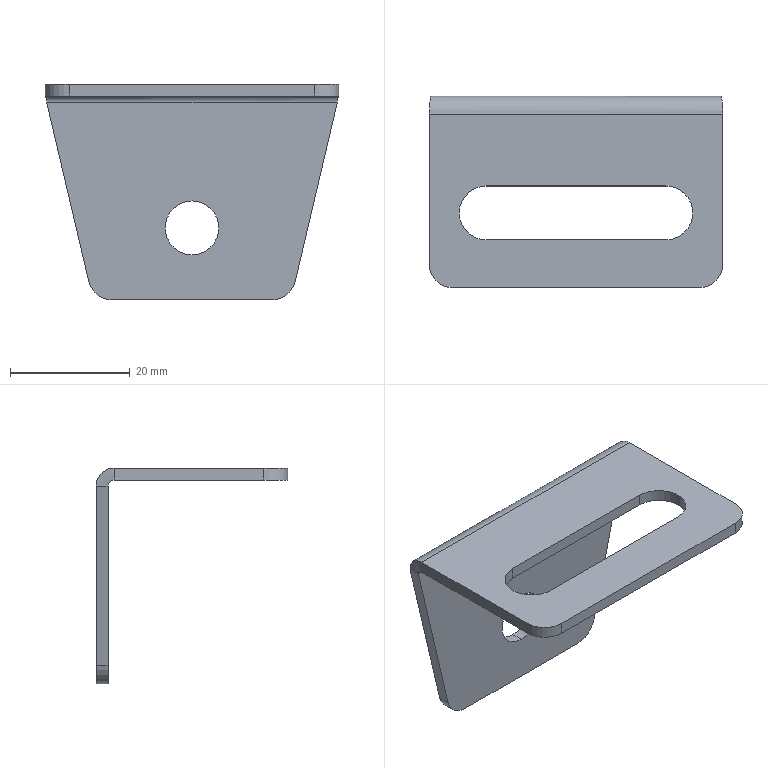Part | STEP file | 1.6米托片 | 1 solid | 25 faces | box 49 x 32 x 36 mm | volume 5023 mm3 | plane 12 | cylinder 11 | spline 2 | commonest cylinder face diameters 9 x5 8 x4 2 x1 6 x1
STEP:
#1=CARTESIAN_POINT('',(5.,12.5,2.));
#2=VERTEX_POINT('',#1);
#3=CARTESIAN_POINT('',(9.5,17.,2.));
#4=VERTEX_POINT('',#3);
#5=CARTESIAN_POINT('',(9.5,12.5,2.));
#6=DIRECTION('',(0.,0.,-1.));
#7=DIRECTION('',(-1.,0.,0.));
#8=AXIS2_PLACEMENT_3D('',#5,#6,#7);
#9=CIRCLE('',#8,4.5);
#10=EDGE_CURVE('',#2,#4,#9,.T.);
#11=ORIENTED_EDGE('',*,*,#10,.F.);
#12=CARTESIAN_POINT('',(5.,12.5,0.));
#13=VERTEX_POINT('',#12);
#14=CARTESIAN_POINT('',(5.,12.5,10.));
#15=DIRECTION('',(0.,0.,-1.));
#16=VECTOR('',#15,1000.);
#17=LINE('',#14,#16);
#18=EDGE_CURVE('',#2,#13,#17,.T.);
#19=ORIENTED_EDGE('',*,*,#18,.T.);
#20=CARTESIAN_POINT('',(9.5,17.,0.));
#21=VERTEX_POINT('',#20);
#22=CARTESIAN_POINT('',(9.5,12.5,0.));
#23=DIRECTION('',(0.,0.,-1.));
#24=DIRECTION('',(-1.,0.,0.));
#25=AXIS2_PLACEMENT_3D('',#22,#23,#24);
#26=CIRCLE('',#25,4.5);
#27=EDGE_CURVE('',#13,#21,#26,.T.);
#28=ORIENTED_EDGE('',*,*,#27,.T.);
#29=CARTESIAN_POINT('',(9.5,17.,10.));
#30=DIRECTION('',(0.,0.,-1.));
#31=VECTOR('',#30,1000.);
#32=LINE('',#29,#31);
#33=EDGE_CURVE('',#4,#21,#32,.T.);
#34=ORIENTED_EDGE('',*,*,#33,.F.);
#35=EDGE_LOOP('',(#11,#19,#28,#34));
#36=FACE_OUTER_BOUND('',#35,.T.);
#37=CARTESIAN_POINT('',(9.5,12.5,10.));
#38=DIRECTION('',(0.,0.,-1.));
#39=DIRECTION('',(-1.,0.,0.));
#40=AXIS2_PLACEMENT_3D('',#37,#38,#39);
#41=CYLINDRICAL_SURFACE('',#40,4.5);
#42=ADVANCED_FACE('',(#36),#41,.F.);
#43=CARTESIAN_POINT('',(24.5,32.,-17.5));
#44=VERTEX_POINT('',#43);
#45=CARTESIAN_POINT('',(24.5,32.,-26.5));
#46=VERTEX_POINT('',#45);
#47=CARTESIAN_POINT('',(24.5,32.,-22.));
#48=DIRECTION('',(0.,-1.,0.));
#49=DIRECTION('',(0.,0.,-1.));
#50=AXIS2_PLACEMENT_3D('',#47,#48,#49);
#51=CIRCLE('',#50,4.5);
#52=EDGE_CURVE('',#44,#46,#51,.T.);
#53=ORIENTED_EDGE('',*,*,#52,.F.);
#54=CARTESIAN_POINT('',(24.5,30.,-17.5));
#55=VERTEX_POINT('',#54);
#56=CARTESIAN_POINT('',(24.5,40.,-17.5));
#57=DIRECTION('',(0.,-1.,0.));
#58=VECTOR('',#57,1000.);
#59=LINE('',#56,#58);
#60=EDGE_CURVE('',#44,#55,#59,.T.);
#61=ORIENTED_EDGE('',*,*,#60,.T.);
#62=CARTESIAN_POINT('',(24.5,30.,-26.5));
#63=VERTEX_POINT('',#62);
#64=CARTESIAN_POINT('',(24.5,30.,-22.));
#65=DIRECTION('',(0.,-1.,0.));
#66=DIRECTION('',(0.,0.,-1.));
#67=AXIS2_PLACEMENT_3D('',#64,#65,#66);
#68=CIRCLE('',#67,4.5);
#69=EDGE_CURVE('',#55,#63,#68,.T.);
#70=ORIENTED_EDGE('',*,*,#69,.T.);
#71=CARTESIAN_POINT('',(24.5,40.,-26.5));
#72=DIRECTION('',(0.,-1.,0.));
#73=VECTOR('',#72,1000.);
#74=LINE('',#71,#73);
#75=EDGE_CURVE('',#46,#63,#74,.T.);
#76=ORIENTED_EDGE('',*,*,#75,.F.);
#77=EDGE_LOOP('',(#53,#61,#70,#76));
#78=FACE_OUTER_BOUND('',#77,.T.);
#79=CARTESIAN_POINT('',(24.5,40.,-22.));
#80=DIRECTION('',(0.,-1.,0.));
#81=DIRECTION('',(0.,0.,-1.));
#82=AXIS2_PLACEMENT_3D('',#79,#80,#81);
#83=CYLINDRICAL_SURFACE('',#82,4.5);
#84=ADVANCED_FACE('',(#78),#83,.F.);
#85=CARTESIAN_POINT('',(39.5,17.,2.));
#86=VERTEX_POINT('',#85);
#87=CARTESIAN_POINT('',(0.,17.,2.));
#88=DIRECTION('',(1.,0.,0.));
#89=VECTOR('',#88,1000.);
#90=LINE('',#87,#89);
#91=EDGE_CURVE('',#4,#86,#90,.T.);
#92=ORIENTED_EDGE('',*,*,#91,.T.);
#93=CARTESIAN_POINT('',(39.5,8.,2.));
#94=VERTEX_POINT('',#93);
#95=CARTESIAN_POINT('',(39.5,12.5,2.));
#96=DIRECTION('',(0.,0.,-1.));
#97=DIRECTION('',(-1.,0.,0.));
#98=AXIS2_PLACEMENT_3D('',#95,#96,#97);
#99=CIRCLE('',#98,4.5);
#100=EDGE_CURVE('',#86,#94,#99,.T.);
#101=ORIENTED_EDGE('',*,*,#100,.T.);
#102=CARTESIAN_POINT('',(9.5,8.,2.));
#103=VERTEX_POINT('',#102);
#104=CARTESIAN_POINT('',(0.,8.,2.));
#105=DIRECTION('',(-1.,0.,0.));
#106=VECTOR('',#105,1000.);
#107=LINE('',#104,#106);
#108=EDGE_CURVE('',#94,#103,#107,.T.);
#109=ORIENTED_EDGE('',*,*,#108,.T.);
#110=CARTESIAN_POINT('',(9.5,12.5,2.));
#111=DIRECTION('',(0.,0.,-1.));
#112=DIRECTION('',(-1.,0.,0.));
#113=AXIS2_PLACEMENT_3D('',#110,#111,#112);
#114=CIRCLE('',#113,4.5);
#115=EDGE_CURVE('',#103,#2,#114,.T.);
#116=ORIENTED_EDGE('',*,*,#115,.T.);
#117=ORIENTED_EDGE('',*,*,#10,.T.);
#118=EDGE_LOOP('',(#92,#101,#109,#116,#117));
#119=FACE_BOUND('',#118,.T.);
#120=CARTESIAN_POINT('',(4.,0.,2.));
#121=VERTEX_POINT('',#120);
#122=CARTESIAN_POINT('',(45.,0.,2.));
#123=VERTEX_POINT('',#122);
#124=CARTESIAN_POINT('',(0.,0.,2.));
#125=DIRECTION('',(1.,0.,0.));
#126=VECTOR('',#125,1000.);
#127=LINE('',#124,#126);
#128=EDGE_CURVE('',#121,#123,#127,.T.);
#129=ORIENTED_EDGE('',*,*,#128,.T.);
#130=CARTESIAN_POINT('',(49.,4.,2.));
#131=VERTEX_POINT('',#130);
#132=CARTESIAN_POINT('',(45.,4.,2.));
#133=DIRECTION('',(0.,0.,1.));
#134=DIRECTION('',(-1.,0.,0.));
#135=AXIS2_PLACEMENT_3D('',#132,#133,#134);
#136=CIRCLE('',#135,4.);
#137=EDGE_CURVE('',#123,#131,#136,.T.);
#138=ORIENTED_EDGE('',*,*,#137,.T.);
#139=CARTESIAN_POINT('',(49.,29.,2.));
#140=VERTEX_POINT('',#139);
#141=CARTESIAN_POINT('',(49.,32.,2.));
#142=DIRECTION('',(0.,-1.,0.));
#143=VECTOR('',#142,1000.);
#144=LINE('',#141,#143);
#145=EDGE_CURVE('',#140,#131,#144,.T.);
#146=ORIENTED_EDGE('',*,*,#145,.F.);
#147=CARTESIAN_POINT('',(0.,29.,2.));
#148=VERTEX_POINT('',#147);
#149=CARTESIAN_POINT('',(49.,29.,2.));
#150=DIRECTION('',(-1.,0.,0.));
#151=VECTOR('',#150,1000.);
#152=LINE('',#149,#151);
#153=EDGE_CURVE('',#140,#148,#152,.T.);
#154=ORIENTED_EDGE('',*,*,#153,.T.);
#155=CARTESIAN_POINT('',(0.,4.,2.));
#156=VERTEX_POINT('',#155);
#157=CARTESIAN_POINT('',(0.,32.,2.));
#158=DIRECTION('',(0.,-1.,0.));
#159=VECTOR('',#158,1000.);
#160=LINE('',#157,#159);
#161=EDGE_CURVE('',#148,#156,#160,.T.);
#162=ORIENTED_EDGE('',*,*,#161,.T.);
#163=CARTESIAN_POINT('',(4.,4.,2.));
#164=DIRECTION('',(0.,0.,1.));
#165=DIRECTION('',(-1.,0.,0.));
#166=AXIS2_PLACEMENT_3D('',#163,#164,#165);
#167=CIRCLE('',#166,4.);
#168=EDGE_CURVE('',#156,#121,#167,.T.);
#169=ORIENTED_EDGE('',*,*,#168,.T.);
#170=EDGE_LOOP('',(#129,#138,#146,#154,#162,#169));
#171=FACE_OUTER_BOUND('',#170,.T.);
#172=CARTESIAN_POINT('',(0.,32.,2.));
#173=DIRECTION('',(0.,0.,-1.));
#174=DIRECTION('',(-1.,0.,0.));
#175=AXIS2_PLACEMENT_3D('',#172,#173,#174);
#176=PLANE('',#175);
#177=ADVANCED_FACE('',(#119,#171),#176,.F.);
#178=ORIENTED_EDGE('',*,*,#145,.T.);
#179=CARTESIAN_POINT('',(49.,4.,0.));
#180=VERTEX_POINT('',#179);
#181=CARTESIAN_POINT('',(49.,4.,0.));
#182=DIRECTION('',(0.,0.,-1.));
#183=VECTOR('',#182,1000.);
#184=LINE('',#181,#183);
#185=EDGE_CURVE('',#131,#180,#184,.T.);
#186=ORIENTED_EDGE('',*,*,#185,.T.);
#187=CARTESIAN_POINT('',(49.,29.,0.));
#188=VERTEX_POINT('',#187);
#189=CARTESIAN_POINT('',(49.,32.,0.));
#190=DIRECTION('',(0.,-1.,0.));
#191=VECTOR('',#190,1000.);
#192=LINE('',#189,#191);
#193=EDGE_CURVE('',#188,#180,#192,.T.);
#194=ORIENTED_EDGE('',*,*,#193,.F.);
#195=CARTESIAN_POINT('',(49.,29.,0.));
#196=DIRECTION('',(0.,0.,1.));
#197=VECTOR('',#196,1000.);
#198=LINE('',#195,#197);
#199=EDGE_CURVE('',#188,#140,#198,.T.);
#200=ORIENTED_EDGE('',*,*,#199,.T.);
#201=EDGE_LOOP('',(#178,#186,#194,#200));
#202=FACE_OUTER_BOUND('',#201,.T.);
#203=CARTESIAN_POINT('',(49.,32.,0.));
#204=DIRECTION('',(1.,0.,0.));
#205=DIRECTION('',(0.,0.,-1.));
#206=AXIS2_PLACEMENT_3D('',#203,#204,#205);
#207=PLANE('',#206);
#208=ADVANCED_FACE('',(#202),#207,.T.);
#209=CARTESIAN_POINT('',(39.5,17.,0.));
#210=VERTEX_POINT('',#209);
#211=CARTESIAN_POINT('',(39.5,8.,0.));
#212=VERTEX_POINT('',#211);
#213=CARTESIAN_POINT('',(39.5,12.5,0.));
#214=DIRECTION('',(0.,0.,-1.));
#215=DIRECTION('',(-1.,0.,0.));
#216=AXIS2_PLACEMENT_3D('',#213,#214,#215);
#217=CIRCLE('',#216,4.5);
#218=EDGE_CURVE('',#210,#212,#217,.T.);
#219=ORIENTED_EDGE('',*,*,#218,.F.);
#220=CARTESIAN_POINT('',(39.5,17.,0.));
#221=DIRECTION('',(1.,0.,0.));
#222=VECTOR('',#221,1000.);
#223=LINE('',#220,#222);
#224=EDGE_CURVE('',#21,#210,#223,.T.);
#225=ORIENTED_EDGE('',*,*,#224,.F.);
#226=ORIENTED_EDGE('',*,*,#27,.F.);
#227=CARTESIAN_POINT('',(9.5,8.,0.));
#228=VERTEX_POINT('',#227);
#229=CARTESIAN_POINT('',(9.5,12.5,0.));
#230=DIRECTION('',(0.,0.,-1.));
#231=DIRECTION('',(-1.,0.,0.));
#232=AXIS2_PLACEMENT_3D('',#229,#230,#231);
#233=CIRCLE('',#232,4.5);
#234=EDGE_CURVE('',#228,#13,#233,.T.);
#235=ORIENTED_EDGE('',*,*,#234,.F.);
#236=CARTESIAN_POINT('',(39.5,8.,0.));
#237=DIRECTION('',(-1.,0.,0.));
#238=VECTOR('',#237,1000.);
#239=LINE('',#236,#238);
#240=EDGE_CURVE('',#212,#228,#239,.T.);
#241=ORIENTED_EDGE('',*,*,#240,.F.);
#242=EDGE_LOOP('',(#219,#225,#226,#235,#241));
#243=FACE_BOUND('',#242,.T.);
#244=ORIENTED_EDGE('',*,*,#193,.T.);
#245=CARTESIAN_POINT('',(45.,0.,0.));
#246=VERTEX_POINT('',#245);
#247=CARTESIAN_POINT('',(45.,4.,0.));
#248=DIRECTION('',(0.,0.,-1.));
#249=DIRECTION('',(-1.,0.,0.));
#250=AXIS2_PLACEMENT_3D('',#247,#248,#249);
#251=CIRCLE('',#250,4.);
#252=EDGE_CURVE('',#180,#246,#251,.T.);
#253=ORIENTED_EDGE('',*,*,#252,.T.);
#254=CARTESIAN_POINT('',(4.,0.,0.));
#255=VERTEX_POINT('',#254);
#256=CARTESIAN_POINT('',(0.,0.,0.));
#257=DIRECTION('',(1.,0.,0.));
#258=VECTOR('',#257,1000.);
#259=LINE('',#256,#258);
#260=EDGE_CURVE('',#255,#246,#259,.T.);
#261=ORIENTED_EDGE('',*,*,#260,.F.);
#262=CARTESIAN_POINT('',(0.,4.,0.));
#263=VERTEX_POINT('',#262);
#264=CARTESIAN_POINT('',(4.,4.,0.));
#265=DIRECTION('',(0.,0.,-1.));
#266=DIRECTION('',(-1.,0.,0.));
#267=AXIS2_PLACEMENT_3D('',#264,#265,#266);
#268=CIRCLE('',#267,4.);
#269=EDGE_CURVE('',#255,#263,#268,.T.);
#270=ORIENTED_EDGE('',*,*,#269,.T.);
#271=CARTESIAN_POINT('',(0.,29.,0.));
#272=VERTEX_POINT('',#271);
#273=CARTESIAN_POINT('',(0.,32.,0.));
#274=DIRECTION('',(0.,-1.,0.));
#275=VECTOR('',#274,1000.);
#276=LINE('',#273,#275);
#277=EDGE_CURVE('',#272,#263,#276,.T.);
#278=ORIENTED_EDGE('',*,*,#277,.F.);
#279=CARTESIAN_POINT('',(49.,29.,0.));
#280=DIRECTION('',(-1.,0.,0.));
#281=VECTOR('',#280,1000.);
#282=LINE('',#279,#281);
#283=EDGE_CURVE('',#188,#272,#282,.T.);
#284=ORIENTED_EDGE('',*,*,#283,.F.);
#285=EDGE_LOOP('',(#244,#253,#261,#270,#278,#284));
#286=FACE_OUTER_BOUND('',#285,.T.);
#287=CARTESIAN_POINT('',(0.,32.,0.));
#288=DIRECTION('',(0.,0.,-1.));
#289=DIRECTION('',(-1.,0.,0.));
#290=AXIS2_PLACEMENT_3D('',#287,#288,#289);
#291=PLANE('',#290);
#292=ADVANCED_FACE('',(#243,#286),#291,.T.);
#293=ORIENTED_EDGE('',*,*,#277,.T.);
#294=CARTESIAN_POINT('',(0.,4.,2.));
#295=DIRECTION('',(0.,0.,1.));
#296=VECTOR('',#295,1000.);
#297=LINE('',#294,#296);
#298=EDGE_CURVE('',#263,#156,#297,.T.);
#299=ORIENTED_EDGE('',*,*,#298,.T.);
#300=ORIENTED_EDGE('',*,*,#161,.F.);
#301=CARTESIAN_POINT('',(0.,29.,0.));
#302=DIRECTION('',(0.,0.,1.));
#303=VECTOR('',#302,1000.);
#304=LINE('',#301,#303);
#305=EDGE_CURVE('',#272,#148,#304,.T.);
#306=ORIENTED_EDGE('',*,*,#305,.F.);
#307=EDGE_LOOP('',(#293,#299,#300,#306));
#308=FACE_OUTER_BOUND('',#307,.T.);
#309=CARTESIAN_POINT('',(0.,32.,2.));
#310=DIRECTION('',(-1.,0.,0.));
#311=DIRECTION('',(0.,0.,1.));
#312=AXIS2_PLACEMENT_3D('',#309,#310,#311);
#313=PLANE('',#312);
#314=ADVANCED_FACE('',(#308),#313,.T.);
#315=ORIENTED_EDGE('',*,*,#260,.T.);
#316=CARTESIAN_POINT('',(45.,0.,0.));
#317=DIRECTION('',(0.,0.,1.));
#318=VECTOR('',#317,1000.);
#319=LINE('',#316,#318);
#320=EDGE_CURVE('',#246,#123,#319,.T.);
#321=ORIENTED_EDGE('',*,*,#320,.T.);
#322=ORIENTED_EDGE('',*,*,#128,.F.);
#323=CARTESIAN_POINT('',(4.,0.,0.));
#324=DIRECTION('',(0.,0.,-1.));
#325=VECTOR('',#324,1000.);
#326=LINE('',#323,#325);
#327=EDGE_CURVE('',#121,#255,#326,.T.);
#328=ORIENTED_EDGE('',*,*,#327,.T.);
#329=EDGE_LOOP('',(#315,#321,#322,#328));
#330=FACE_OUTER_BOUND('',#329,.T.);
#331=CARTESIAN_POINT('',(0.,0.,0.));
#332=DIRECTION('',(0.,-1.,0.));
#333=DIRECTION('',(-1.,0.,0.));
#334=AXIS2_PLACEMENT_3D('',#331,#332,#333);
#335=PLANE('',#334);
#336=ADVANCED_FACE('',(#330),#335,.T.);
#337=CARTESIAN_POINT('',(0.2353,30.,-1.));
#338=VERTEX_POINT('',#337);
#339=CARTESIAN_POINT('',(0.2353,32.,-1.));
#340=VERTEX_POINT('',#339);
#341=CARTESIAN_POINT('',(0.2353,32.,-1.));
#342=DIRECTION('',(0.,1.,0.));
#343=VECTOR('',#342,1000.);
#344=LINE('',#341,#343);
#345=EDGE_CURVE('',#338,#340,#344,.T.);
#346=ORIENTED_EDGE('',*,*,#345,.F.);
#347=CARTESIAN_POINT('',(0.,29.,0.));
#348=CARTESIAN_POINT('',(0.03922,29.262,0.));
#349=CARTESIAN_POINT('',(0.07843,29.522,-0.1078));
#350=CARTESIAN_POINT('',(0.1569,29.892,-0.478));
#351=CARTESIAN_POINT('',(0.1961,30.,-0.7382));
#352=CARTESIAN_POINT('',(0.2353,30.,-1.));
#353=B_SPLINE_CURVE_WITH_KNOTS('',3,(#347,#348,#349,#350,#351,#352),.UNSPECIFIED.,.F.,.F.,(4,2,4),(0.,0.5,1.),.UNSPECIFIED.);
#354=EDGE_CURVE('',#272,#338,#353,.T.);
#355=ORIENTED_EDGE('',*,*,#354,.F.);
#356=ORIENTED_EDGE('',*,*,#305,.T.);
#357=CARTESIAN_POINT('',(0.,29.,2.));
#358=CARTESIAN_POINT('',(0.01961,29.393,2.));
#359=CARTESIAN_POINT('',(0.03922,29.785,1.922));
#360=CARTESIAN_POINT('',(0.07843,30.511,1.621));
#361=CARTESIAN_POINT('',(0.09804,30.844,1.399));
#362=CARTESIAN_POINT('',(0.1373,31.399,0.8436));
#363=CARTESIAN_POINT('',(0.1569,31.621,0.5109));
#364=CARTESIAN_POINT('',(0.1961,31.922,-0.2148));
#365=CARTESIAN_POINT('',(0.2157,32.,-0.6073));
#366=CARTESIAN_POINT('',(0.2353,32.,-1.));
#367=B_SPLINE_CURVE_WITH_KNOTS('',3,(#357,#358,#359,#360,#361,#362,#363,#364,#365,#366),.UNSPECIFIED.,.F.,.F.,(4,2,2,2,4),(0.,0.25,0.5,0.75,1.),.UNSPECIFIED.);
#368=EDGE_CURVE('',#148,#340,#367,.T.);
#369=ORIENTED_EDGE('',*,*,#368,.T.);
#370=EDGE_LOOP('',(#346,#355,#356,#369));
#371=FACE_OUTER_BOUND('',#370,.T.);
#372=CARTESIAN_POINT('',(0.,29.,2.02));
#373=CARTESIAN_POINT('',(0.01961,29.395,2.02));
#374=CARTESIAN_POINT('',(0.03922,29.79,1.941));
#375=CARTESIAN_POINT('',(0.07843,30.521,1.639));
#376=CARTESIAN_POINT('',(0.09804,30.856,1.415));
#377=CARTESIAN_POINT('',(0.1373,31.415,0.8559));
#378=CARTESIAN_POINT('',(0.1569,31.639,0.5209));
#379=CARTESIAN_POINT('',(0.1961,31.941,-0.2095));
#380=CARTESIAN_POINT('',(0.2157,32.02,-0.6046));
#381=CARTESIAN_POINT('',(0.2353,32.02,-1.));
#382=CARTESIAN_POINT('',(0.,29.,2.));
#383=CARTESIAN_POINT('',(0.01961,29.393,2.));
#384=CARTESIAN_POINT('',(0.03922,29.785,1.922));
#385=CARTESIAN_POINT('',(0.07843,30.511,1.621));
#386=CARTESIAN_POINT('',(0.09804,30.844,1.399));
#387=CARTESIAN_POINT('',(0.1373,31.399,0.8436));
#388=CARTESIAN_POINT('',(0.1569,31.621,0.5109));
#389=CARTESIAN_POINT('',(0.1961,31.922,-0.2148));
#390=CARTESIAN_POINT('',(0.2157,32.,-0.6072));
#391=CARTESIAN_POINT('',(0.2353,32.,-1.));
#392=CARTESIAN_POINT('',(0.,29.,0.));
#393=CARTESIAN_POINT('',(0.01961,29.131,0.));
#394=CARTESIAN_POINT('',(0.03922,29.262,-0.02603));
#395=CARTESIAN_POINT('',(0.07843,29.504,-0.1262));
#396=CARTESIAN_POINT('',(0.09804,29.615,-0.2003));
#397=CARTESIAN_POINT('',(0.1373,29.8,-0.3855));
#398=CARTESIAN_POINT('',(0.1569,29.874,-0.4964));
#399=CARTESIAN_POINT('',(0.1961,29.974,-0.7383));
#400=CARTESIAN_POINT('',(0.2157,30.,-0.8691));
#401=CARTESIAN_POINT('',(0.2353,30.,-1.));
#402=CARTESIAN_POINT('',(0.,29.,-0.0202));
#403=CARTESIAN_POINT('',(0.01961,29.128,-0.0202));
#404=CARTESIAN_POINT('',(0.03922,29.256,-0.0457));
#405=CARTESIAN_POINT('',(0.07843,29.493,-0.1439));
#406=CARTESIAN_POINT('',(0.09804,29.602,-0.2165));
#407=CARTESIAN_POINT('',(0.1373,29.784,-0.3979));
#408=CARTESIAN_POINT('',(0.1569,29.856,-0.5066));
#409=CARTESIAN_POINT('',(0.1961,29.954,-0.7435));
#410=CARTESIAN_POINT('',(0.2157,29.98,-0.8717));
#411=CARTESIAN_POINT('',(0.2353,29.98,-1.));
#412=B_SPLINE_SURFACE_WITH_KNOTS('',1,3,((#372,#373,#374,#375,#376,#377,#378,#379,#380,#381),(#382,#383,#384,#385,#386,#387,#388,#389,#390,#391),(#392,#393,#394,#395,#396,#397,#398,#399,#400,#401),(#402,#403,#404,#405,#406,#407,#408,#409,#410,#411)),.UNSPECIFIED.,.F.,.F.,.F.,(2,1,1,2),(4,2,2,2,4),(-0.01,0.,1.,1.01),(0.,0.25,0.5,0.75,1.),.UNSPECIFIED.);
#413=ADVANCED_FACE('',(#371),#412,.F.);
#414=CARTESIAN_POINT('',(48.765,30.,-1.));
#415=VERTEX_POINT('',#414);
#416=CARTESIAN_POINT('',(48.765,30.,-1.));
#417=CARTESIAN_POINT('',(48.804,30.,-0.7382));
#418=CARTESIAN_POINT('',(48.843,29.892,-0.478));
#419=CARTESIAN_POINT('',(48.922,29.522,-0.1078));
#420=CARTESIAN_POINT('',(48.961,29.262,0.));
#421=CARTESIAN_POINT('',(49.,29.,0.));
#422=B_SPLINE_CURVE_WITH_KNOTS('',3,(#416,#417,#418,#419,#420,#421),.UNSPECIFIED.,.F.,.F.,(4,2,4),(0.,0.5,1.),.UNSPECIFIED.);
#423=EDGE_CURVE('',#415,#188,#422,.T.);
#424=ORIENTED_EDGE('',*,*,#423,.F.);
#425=CARTESIAN_POINT('',(48.765,32.,-1.));
#426=VERTEX_POINT('',#425);
#427=CARTESIAN_POINT('',(48.765,30.,-1.));
#428=DIRECTION('',(0.,1.,0.));
#429=VECTOR('',#428,1000.);
#430=LINE('',#427,#429);
#431=EDGE_CURVE('',#415,#426,#430,.T.);
#432=ORIENTED_EDGE('',*,*,#431,.T.);
#433=CARTESIAN_POINT('',(48.765,32.,-1.));
#434=CARTESIAN_POINT('',(48.784,32.,-0.6073));
#435=CARTESIAN_POINT('',(48.804,31.922,-0.2148));
#436=CARTESIAN_POINT('',(48.843,31.621,0.5109));
#437=CARTESIAN_POINT('',(48.863,31.399,0.8436));
#438=CARTESIAN_POINT('',(48.902,30.844,1.399));
#439=CARTESIAN_POINT('',(48.922,30.511,1.621));
#440=CARTESIAN_POINT('',(48.961,29.785,1.922));
#441=CARTESIAN_POINT('',(48.98,29.393,2.));
#442=CARTESIAN_POINT('',(49.,29.,2.));
#443=B_SPLINE_CURVE_WITH_KNOTS('',3,(#433,#434,#435,#436,#437,#438,#439,#440,#441,#442),.UNSPECIFIED.,.F.,.F.,(4,2,2,2,4),(0.,0.25,0.5,0.75,1.),.UNSPECIFIED.);
#444=EDGE_CURVE('',#426,#140,#443,.T.);
#445=ORIENTED_EDGE('',*,*,#444,.T.);
#446=ORIENTED_EDGE('',*,*,#199,.F.);
#447=EDGE_LOOP('',(#424,#432,#445,#446));
#448=FACE_OUTER_BOUND('',#447,.T.);
#449=CARTESIAN_POINT('',(48.765,32.02,-1.));
#450=CARTESIAN_POINT('',(48.784,32.02,-0.6046));
#451=CARTESIAN_POINT('',(48.804,31.941,-0.2095));
#452=CARTESIAN_POINT('',(48.843,31.639,0.5209));
#453=CARTESIAN_POINT('',(48.863,31.415,0.8559));
#454=CARTESIAN_POINT('',(48.902,30.856,1.415));
#455=CARTESIAN_POINT('',(48.922,30.521,1.639));
#456=CARTESIAN_POINT('',(48.961,29.79,1.941));
#457=CARTESIAN_POINT('',(48.98,29.395,2.02));
#458=CARTESIAN_POINT('',(49.,29.,2.02));
#459=CARTESIAN_POINT('',(48.765,32.,-1.));
#460=CARTESIAN_POINT('',(48.784,32.,-0.6072));
#461=CARTESIAN_POINT('',(48.804,31.922,-0.2148));
#462=CARTESIAN_POINT('',(48.843,31.621,0.5109));
#463=CARTESIAN_POINT('',(48.863,31.399,0.8436));
#464=CARTESIAN_POINT('',(48.902,30.844,1.399));
#465=CARTESIAN_POINT('',(48.922,30.511,1.621));
#466=CARTESIAN_POINT('',(48.961,29.785,1.922));
#467=CARTESIAN_POINT('',(48.98,29.393,2.));
#468=CARTESIAN_POINT('',(49.,29.,2.));
#469=CARTESIAN_POINT('',(48.765,30.,-1.));
#470=CARTESIAN_POINT('',(48.784,30.,-0.8691));
#471=CARTESIAN_POINT('',(48.804,29.974,-0.7383));
#472=CARTESIAN_POINT('',(48.843,29.874,-0.4964));
#473=CARTESIAN_POINT('',(48.863,29.8,-0.3855));
#474=CARTESIAN_POINT('',(48.902,29.615,-0.2003));
#475=CARTESIAN_POINT('',(48.922,29.504,-0.1262));
#476=CARTESIAN_POINT('',(48.961,29.262,-0.02603));
#477=CARTESIAN_POINT('',(48.98,29.131,0.));
#478=CARTESIAN_POINT('',(49.,29.,0.));
#479=CARTESIAN_POINT('',(48.765,29.98,-1.));
#480=CARTESIAN_POINT('',(48.784,29.98,-0.8717));
#481=CARTESIAN_POINT('',(48.804,29.954,-0.7435));
#482=CARTESIAN_POINT('',(48.843,29.856,-0.5066));
#483=CARTESIAN_POINT('',(48.863,29.784,-0.3979));
#484=CARTESIAN_POINT('',(48.902,29.602,-0.2165));
#485=CARTESIAN_POINT('',(48.922,29.493,-0.1439));
#486=CARTESIAN_POINT('',(48.961,29.256,-0.0457));
#487=CARTESIAN_POINT('',(48.98,29.128,-0.0202));
#488=CARTESIAN_POINT('',(49.,29.,-0.0202));
#489=B_SPLINE_SURFACE_WITH_KNOTS('',1,3,((#449,#450,#451,#452,#453,#454,#455,#456,#457,#458),(#459,#460,#461,#462,#463,#464,#465,#466,#467,#468),(#469,#470,#471,#472,#473,#474,#475,#476,#477,#478),(#479,#480,#481,#482,#483,#484,#485,#486,#487,#488)),.UNSPECIFIED.,.F.,.F.,.F.,(2,1,1,2),(4,2,2,2,4),(-0.01,0.,1.,1.01),(0.,0.25,0.5,0.75,1.),.UNSPECIFIED.);
#490=ADVANCED_FACE('',(#448),#489,.F.);
#491=ORIENTED_EDGE('',*,*,#153,.F.);
#492=ORIENTED_EDGE('',*,*,#444,.F.);
#493=CARTESIAN_POINT('',(0.2353,32.,-1.));
#494=DIRECTION('',(-1.,0.,0.));
#495=VECTOR('',#494,1000.);
#496=LINE('',#493,#495);
#497=EDGE_CURVE('',#426,#340,#496,.T.);
#498=ORIENTED_EDGE('',*,*,#497,.T.);
#499=ORIENTED_EDGE('',*,*,#368,.F.);
#500=EDGE_LOOP('',(#491,#492,#498,#499));
#501=FACE_OUTER_BOUND('',#500,.T.);
#502=CARTESIAN_POINT('',(49.,29.,-1.));
#503=DIRECTION('',(1.,0.,0.));
#504=DIRECTION('',(0.,1.,0.));
#505=AXIS2_PLACEMENT_3D('',#502,#503,#504);
#506=CYLINDRICAL_SURFACE('',#505,3.);
#507=ADVANCED_FACE('',(#501),#506,.T.);
#508=ORIENTED_EDGE('',*,*,#283,.T.);
#509=ORIENTED_EDGE('',*,*,#354,.T.);
#510=CARTESIAN_POINT('',(0.2353,30.,-1.));
#511=DIRECTION('',(1.,0.,0.));
#512=VECTOR('',#511,1000.);
#513=LINE('',#510,#512);
#514=EDGE_CURVE('',#338,#415,#513,.T.);
#515=ORIENTED_EDGE('',*,*,#514,.T.);
#516=ORIENTED_EDGE('',*,*,#423,.T.);
#517=EDGE_LOOP('',(#508,#509,#515,#516));
#518=FACE_OUTER_BOUND('',#517,.T.);
#519=CARTESIAN_POINT('',(49.,29.,-1.));
#520=DIRECTION('',(1.,0.,0.));
#521=DIRECTION('',(0.,1.,0.));
#522=AXIS2_PLACEMENT_3D('',#519,#520,#521);
#523=CYLINDRICAL_SURFACE('',#522,1.);
#524=ADVANCED_FACE('',(#518),#523,.F.);
#525=CARTESIAN_POINT('',(7.274,32.,-30.916));
#526=VERTEX_POINT('',#525);
#527=CARTESIAN_POINT('',(0.,32.,0.));
#528=DIRECTION('',(-0.229,0.,0.9734));
#529=VECTOR('',#528,1000.);
#530=LINE('',#527,#529);
#531=EDGE_CURVE('',#526,#340,#530,.T.);
#532=ORIENTED_EDGE('',*,*,#531,.F.);
#533=CARTESIAN_POINT('',(7.274,30.,-30.916));
#534=VERTEX_POINT('',#533);
#535=CARTESIAN_POINT('',(7.274,32.,-30.916));
#536=DIRECTION('',(0.,-1.,0.));
#537=VECTOR('',#536,1000.);
#538=LINE('',#535,#537);
#539=EDGE_CURVE('',#526,#534,#538,.T.);
#540=ORIENTED_EDGE('',*,*,#539,.T.);
#541=CARTESIAN_POINT('',(0.,30.,0.));
#542=DIRECTION('',(-0.229,0.,0.9734));
#543=VECTOR('',#542,1000.);
#544=LINE('',#541,#543);
#545=EDGE_CURVE('',#534,#338,#544,.T.);
#546=ORIENTED_EDGE('',*,*,#545,.T.);
#547=ORIENTED_EDGE('',*,*,#345,.T.);
#548=EDGE_LOOP('',(#532,#540,#546,#547));
#549=FACE_OUTER_BOUND('',#548,.T.);
#550=CARTESIAN_POINT('',(0.,32.,0.));
#551=DIRECTION('',(0.9734,0.,0.229));
#552=DIRECTION('',(0.229,0.,-0.9734));
#553=AXIS2_PLACEMENT_3D('',#550,#551,#552);
#554=PLANE('',#553);
#555=ADVANCED_FACE('',(#549),#554,.F.);
#556=CARTESIAN_POINT('',(41.726,30.,-30.916));
#557=VERTEX_POINT('',#556);
#558=CARTESIAN_POINT('',(49.,30.,0.));
#559=DIRECTION('',(-0.229,0.,-0.9734));
#560=VECTOR('',#559,1000.);
#561=LINE('',#558,#560);
#562=EDGE_CURVE('',#415,#557,#561,.T.);
#563=ORIENTED_EDGE('',*,*,#562,.T.);
#564=CARTESIAN_POINT('',(41.726,32.,-30.916));
#565=VERTEX_POINT('',#564);
#566=CARTESIAN_POINT('',(41.726,32.,-30.916));
#567=DIRECTION('',(0.,1.,0.));
#568=VECTOR('',#567,1000.);
#569=LINE('',#566,#568);
#570=EDGE_CURVE('',#557,#565,#569,.T.);
#571=ORIENTED_EDGE('',*,*,#570,.T.);
#572=CARTESIAN_POINT('',(46.43,32.,-10.925));
#573=DIRECTION('',(-0.229,0.,-0.9734));
#574=VECTOR('',#573,1000.);
#575=LINE('',#572,#574);
#576=EDGE_CURVE('',#426,#565,#575,.T.);
#577=ORIENTED_EDGE('',*,*,#576,.F.);
#578=ORIENTED_EDGE('',*,*,#431,.F.);
#579=EDGE_LOOP('',(#563,#571,#577,#578));
#580=FACE_OUTER_BOUND('',#579,.T.);
#581=CARTESIAN_POINT('',(49.,32.,0.));
#582=DIRECTION('',(-0.9734,0.,0.229));
#583=DIRECTION('',(0.229,0.,0.9734));
#584=AXIS2_PLACEMENT_3D('',#581,#582,#583);
#585=PLANE('',#584);
#586=ADVANCED_FACE('',(#580),#585,.F.);
#587=CARTESIAN_POINT('',(24.5,32.,-22.));
#588=DIRECTION('',(0.,-1.,0.));
#589=DIRECTION('',(0.,0.,-1.));
#590=AXIS2_PLACEMENT_3D('',#587,#588,#589);
#591=CIRCLE('',#590,4.5);
#592=EDGE_CURVE('',#46,#44,#591,.T.);
#593=ORIENTED_EDGE('',*,*,#592,.T.);
#594=ORIENTED_EDGE('',*,*,#52,.T.);
#595=EDGE_LOOP('',(#593,#594));
#596=FACE_BOUND('',#595,.T.);
#597=CARTESIAN_POINT('',(37.832,32.,-34.));
#598=VERTEX_POINT('',#597);
#599=CARTESIAN_POINT('',(11.168,32.,-34.));
#600=VERTEX_POINT('',#599);
#601=CARTESIAN_POINT('',(0.,32.,-34.));
#602=DIRECTION('',(-1.,0.,0.));
#603=VECTOR('',#602,1000.);
#604=LINE('',#601,#603);
#605=EDGE_CURVE('',#598,#600,#604,.T.);
#606=ORIENTED_EDGE('',*,*,#605,.T.);
#607=CARTESIAN_POINT('',(11.168,32.,-30.));
#608=DIRECTION('',(0.,1.,0.));
#609=DIRECTION('',(0.,0.,-1.));
#610=AXIS2_PLACEMENT_3D('',#607,#608,#609);
#611=CIRCLE('',#610,4.);
#612=EDGE_CURVE('',#600,#526,#611,.T.);
#613=ORIENTED_EDGE('',*,*,#612,.T.);
#614=ORIENTED_EDGE('',*,*,#531,.T.);
#615=ORIENTED_EDGE('',*,*,#497,.F.);
#616=ORIENTED_EDGE('',*,*,#576,.T.);
#617=CARTESIAN_POINT('',(37.832,32.,-30.));
#618=DIRECTION('',(0.,1.,0.));
#619=DIRECTION('',(0.,0.,-1.));
#620=AXIS2_PLACEMENT_3D('',#617,#618,#619);
#621=CIRCLE('',#620,4.);
#622=EDGE_CURVE('',#565,#598,#621,.T.);
#623=ORIENTED_EDGE('',*,*,#622,.T.);
#624=EDGE_LOOP('',(#606,#613,#614,#615,#616,#623));
#625=FACE_OUTER_BOUND('',#624,.T.);
#626=CARTESIAN_POINT('',(0.,32.,0.));
#627=DIRECTION('',(0.,-1.,0.));
#628=DIRECTION('',(0.,0.,-1.));
#629=AXIS2_PLACEMENT_3D('',#626,#627,#628);
#630=PLANE('',#629);
#631=ADVANCED_FACE('',(#596,#625),#630,.F.);
#632=CARTESIAN_POINT('',(24.5,30.,-22.));
#633=DIRECTION('',(0.,-1.,0.));
#634=DIRECTION('',(0.,0.,-1.));
#635=AXIS2_PLACEMENT_3D('',#632,#633,#634);
#636=CIRCLE('',#635,4.5);
#637=EDGE_CURVE('',#63,#55,#636,.T.);
#638=ORIENTED_EDGE('',*,*,#637,.F.);
#639=ORIENTED_EDGE('',*,*,#69,.F.);
#640=EDGE_LOOP('',(#638,#639));
#641=FACE_BOUND('',#640,.T.);
#642=ORIENTED_EDGE('',*,*,#545,.F.);
#643=CARTESIAN_POINT('',(11.168,30.,-34.));
#644=VERTEX_POINT('',#643);
#645=CARTESIAN_POINT('',(11.168,30.,-30.));
#646=DIRECTION('',(0.,-1.,0.));
#647=DIRECTION('',(0.,0.,-1.));
#648=AXIS2_PLACEMENT_3D('',#645,#646,#647);
#649=CIRCLE('',#648,4.);
#650=EDGE_CURVE('',#534,#644,#649,.T.);
#651=ORIENTED_EDGE('',*,*,#650,.T.);
#652=CARTESIAN_POINT('',(37.832,30.,-34.));
#653=VERTEX_POINT('',#652);
#654=CARTESIAN_POINT('',(8.,30.,-34.));
#655=DIRECTION('',(-1.,0.,0.));
#656=VECTOR('',#655,1000.);
#657=LINE('',#654,#656);
#658=EDGE_CURVE('',#653,#644,#657,.T.);
#659=ORIENTED_EDGE('',*,*,#658,.F.);
#660=CARTESIAN_POINT('',(37.832,30.,-30.));
#661=DIRECTION('',(0.,-1.,0.));
#662=DIRECTION('',(0.,0.,-1.));
#663=AXIS2_PLACEMENT_3D('',#660,#661,#662);
#664=CIRCLE('',#663,4.);
#665=EDGE_CURVE('',#653,#557,#664,.T.);
#666=ORIENTED_EDGE('',*,*,#665,.T.);
#667=ORIENTED_EDGE('',*,*,#562,.F.);
#668=ORIENTED_EDGE('',*,*,#514,.F.);
#669=EDGE_LOOP('',(#642,#651,#659,#666,#667,#668));
#670=FACE_OUTER_BOUND('',#669,.T.);
#671=CARTESIAN_POINT('',(0.,30.,0.));
#672=DIRECTION('',(0.,-1.,0.));
#673=DIRECTION('',(0.,0.,-1.));
#674=AXIS2_PLACEMENT_3D('',#671,#672,#673);
#675=PLANE('',#674);
#676=ADVANCED_FACE('',(#641,#670),#675,.T.);
#677=ORIENTED_EDGE('',*,*,#658,.T.);
#678=CARTESIAN_POINT('',(11.168,32.,-34.));
#679=DIRECTION('',(0.,1.,0.));
#680=VECTOR('',#679,1000.);
#681=LINE('',#678,#680);
#682=EDGE_CURVE('',#644,#600,#681,.T.);
#683=ORIENTED_EDGE('',*,*,#682,.T.);
#684=ORIENTED_EDGE('',*,*,#605,.F.);
#685=CARTESIAN_POINT('',(37.832,32.,-34.));
#686=DIRECTION('',(0.,-1.,0.));
#687=VECTOR('',#686,1000.);
#688=LINE('',#685,#687);
#689=EDGE_CURVE('',#598,#653,#688,.T.);
#690=ORIENTED_EDGE('',*,*,#689,.T.);
#691=EDGE_LOOP('',(#677,#683,#684,#690));
#692=FACE_OUTER_BOUND('',#691,.T.);
#693=CARTESIAN_POINT('',(8.,32.,-34.));
#694=DIRECTION('',(0.,0.,1.));
#695=DIRECTION('',(0.,-1.,0.));
#696=AXIS2_PLACEMENT_3D('',#693,#694,#695);
#697=PLANE('',#696);
#698=ADVANCED_FACE('',(#692),#697,.F.);
#699=ORIENTED_EDGE('',*,*,#60,.F.);
#700=ORIENTED_EDGE('',*,*,#592,.F.);
#701=ORIENTED_EDGE('',*,*,#75,.T.);
#702=ORIENTED_EDGE('',*,*,#637,.T.);
#703=EDGE_LOOP('',(#699,#700,#701,#702));
#704=FACE_OUTER_BOUND('',#703,.T.);
#705=CARTESIAN_POINT('',(24.5,40.,-22.));
#706=DIRECTION('',(0.,-1.,0.));
#707=DIRECTION('',(0.,0.,-1.));
#708=AXIS2_PLACEMENT_3D('',#705,#706,#707);
#709=CYLINDRICAL_SURFACE('',#708,4.5);
#710=ADVANCED_FACE('',(#704),#709,.F.);
#711=CARTESIAN_POINT('',(39.5,17.,10.));
#712=DIRECTION('',(0.,0.,-1.));
#713=VECTOR('',#712,1000.);
#714=LINE('',#711,#713);
#715=EDGE_CURVE('',#86,#210,#714,.T.);
#716=ORIENTED_EDGE('',*,*,#715,.T.);
#717=ORIENTED_EDGE('',*,*,#218,.T.);
#718=CARTESIAN_POINT('',(39.5,8.,10.));
#719=DIRECTION('',(0.,0.,-1.));
#720=VECTOR('',#719,1000.);
#721=LINE('',#718,#720);
#722=EDGE_CURVE('',#94,#212,#721,.T.);
#723=ORIENTED_EDGE('',*,*,#722,.F.);
#724=ORIENTED_EDGE('',*,*,#100,.F.);
#725=EDGE_LOOP('',(#716,#717,#723,#724));
#726=FACE_OUTER_BOUND('',#725,.T.);
#727=CARTESIAN_POINT('',(39.5,12.5,10.));
#728=DIRECTION('',(0.,0.,-1.));
#729=DIRECTION('',(-1.,0.,0.));
#730=AXIS2_PLACEMENT_3D('',#727,#728,#729);
#731=CYLINDRICAL_SURFACE('',#730,4.5);
#732=ADVANCED_FACE('',(#726),#731,.F.);
#733=ORIENTED_EDGE('',*,*,#33,.T.);
#734=ORIENTED_EDGE('',*,*,#224,.T.);
#735=ORIENTED_EDGE('',*,*,#715,.F.);
#736=ORIENTED_EDGE('',*,*,#91,.F.);
#737=EDGE_LOOP('',(#733,#734,#735,#736));
#738=FACE_OUTER_BOUND('',#737,.T.);
#739=CARTESIAN_POINT('',(39.5,17.,10.));
#740=DIRECTION('',(0.,1.,0.));
#741=DIRECTION('',(0.,0.,1.));
#742=AXIS2_PLACEMENT_3D('',#739,#740,#741);
#743=PLANE('',#742);
#744=ADVANCED_FACE('',(#738),#743,.F.);
#745=ORIENTED_EDGE('',*,*,#18,.F.);
#746=ORIENTED_EDGE('',*,*,#115,.F.);
#747=CARTESIAN_POINT('',(9.5,8.,10.));
#748=DIRECTION('',(0.,0.,-1.));
#749=VECTOR('',#748,1000.);
#750=LINE('',#747,#749);
#751=EDGE_CURVE('',#103,#228,#750,.T.);
#752=ORIENTED_EDGE('',*,*,#751,.T.);
#753=ORIENTED_EDGE('',*,*,#234,.T.);
#754=EDGE_LOOP('',(#745,#746,#752,#753));
#755=FACE_OUTER_BOUND('',#754,.T.);
#756=CARTESIAN_POINT('',(9.5,12.5,10.));
#757=DIRECTION('',(0.,0.,-1.));
#758=DIRECTION('',(-1.,0.,0.));
#759=AXIS2_PLACEMENT_3D('',#756,#757,#758);
#760=CYLINDRICAL_SURFACE('',#759,4.5);
#761=ADVANCED_FACE('',(#755),#760,.F.);
#762=ORIENTED_EDGE('',*,*,#722,.T.);
#763=ORIENTED_EDGE('',*,*,#240,.T.);
#764=ORIENTED_EDGE('',*,*,#751,.F.);
#765=ORIENTED_EDGE('',*,*,#108,.F.);
#766=EDGE_LOOP('',(#762,#763,#764,#765));
#767=FACE_OUTER_BOUND('',#766,.T.);
#768=CARTESIAN_POINT('',(39.5,8.,10.));
#769=DIRECTION('',(0.,-1.,0.));
#770=DIRECTION('',(0.,0.,-1.));
#771=AXIS2_PLACEMENT_3D('',#768,#769,#770);
#772=PLANE('',#771);
#773=ADVANCED_FACE('',(#767),#772,.F.);
#774=ORIENTED_EDGE('',*,*,#612,.F.);
#775=ORIENTED_EDGE('',*,*,#682,.F.);
#776=ORIENTED_EDGE('',*,*,#650,.F.);
#777=ORIENTED_EDGE('',*,*,#539,.F.);
#778=EDGE_LOOP('',(#774,#775,#776,#777));
#779=FACE_OUTER_BOUND('',#778,.T.);
#780=CARTESIAN_POINT('',(11.168,32.,-30.));
#781=DIRECTION('',(0.,-1.,0.));
#782=DIRECTION('',(0.,0.,-1.));
#783=AXIS2_PLACEMENT_3D('',#780,#781,#782);
#784=CYLINDRICAL_SURFACE('',#783,4.);
#785=ADVANCED_FACE('',(#779),#784,.T.);
#786=ORIENTED_EDGE('',*,*,#622,.F.);
#787=ORIENTED_EDGE('',*,*,#570,.F.);
#788=ORIENTED_EDGE('',*,*,#665,.F.);
#789=ORIENTED_EDGE('',*,*,#689,.F.);
#790=EDGE_LOOP('',(#786,#787,#788,#789));
#791=FACE_OUTER_BOUND('',#790,.T.);
#792=CARTESIAN_POINT('',(37.832,32.,-30.));
#793=DIRECTION('',(0.,-1.,0.));
#794=DIRECTION('',(0.,0.,-1.));
#795=AXIS2_PLACEMENT_3D('',#792,#793,#794);
#796=CYLINDRICAL_SURFACE('',#795,4.);
#797=ADVANCED_FACE('',(#791),#796,.T.);
#798=ORIENTED_EDGE('',*,*,#252,.F.);
#799=ORIENTED_EDGE('',*,*,#185,.F.);
#800=ORIENTED_EDGE('',*,*,#137,.F.);
#801=ORIENTED_EDGE('',*,*,#320,.F.);
#802=EDGE_LOOP('',(#798,#799,#800,#801));
#803=FACE_OUTER_BOUND('',#802,.T.);
#804=CARTESIAN_POINT('',(45.,4.,0.));
#805=DIRECTION('',(0.,0.,1.));
#806=DIRECTION('',(1.,0.,0.));
#807=AXIS2_PLACEMENT_3D('',#804,#805,#806);
#808=CYLINDRICAL_SURFACE('',#807,4.);
#809=ADVANCED_FACE('',(#803),#808,.T.);
#810=ORIENTED_EDGE('',*,*,#168,.F.);
#811=ORIENTED_EDGE('',*,*,#298,.F.);
#812=ORIENTED_EDGE('',*,*,#269,.F.);
#813=ORIENTED_EDGE('',*,*,#327,.F.);
#814=EDGE_LOOP('',(#810,#811,#812,#813));
#815=FACE_OUTER_BOUND('',#814,.T.);
#816=CARTESIAN_POINT('',(4.,4.,0.));
#817=DIRECTION('',(0.,0.,-1.));
#818=DIRECTION('',(-1.,0.,0.));
#819=AXIS2_PLACEMENT_3D('',#816,#817,#818);
#820=CYLINDRICAL_SURFACE('',#819,4.);
#821=ADVANCED_FACE('',(#815),#820,.T.);
#822=CLOSED_SHELL('',(#42,#84,#177,#208,#292,#314,#336,#413,#490,#507,#524,#555,#586,#631,#676,#698,#710,#732,#744,#761,#773,#785,#797,#809,#821));
#823=MANIFOLD_SOLID_BREP('',#822);
#824=CARTESIAN_POINT('',(0.,0.,0.));
#825=DIRECTION('',(0.,0.,1.));
#826=DIRECTION('',(1.,0.,0.));
#827=AXIS2_PLACEMENT_3D('',#824,#825,#826);
#828=(LENGTH_UNIT()NAMED_UNIT(*)SI_UNIT(.MILLI.,.METRE.));
#829=UNCERTAINTY_MEASURE_WITH_UNIT(LENGTH_MEASURE(0.00001),#828,'','');
#830=(NAMED_UNIT(*)PLANE_ANGLE_UNIT()SI_UNIT($,.RADIAN.));
#831=(NAMED_UNIT(*)SI_UNIT($,.STERADIAN.)SOLID_ANGLE_UNIT());
#832=(GEOMETRIC_REPRESENTATION_CONTEXT(3)GLOBAL_UNCERTAINTY_ASSIGNED_CONTEXT((#829))GLOBAL_UNIT_ASSIGNED_CONTEXT((#828,#830,#831))REPRESENTATION_CONTEXT('',''));
#833=ADVANCED_BREP_SHAPE_REPRESENTATION('',(#823,#827),#832);